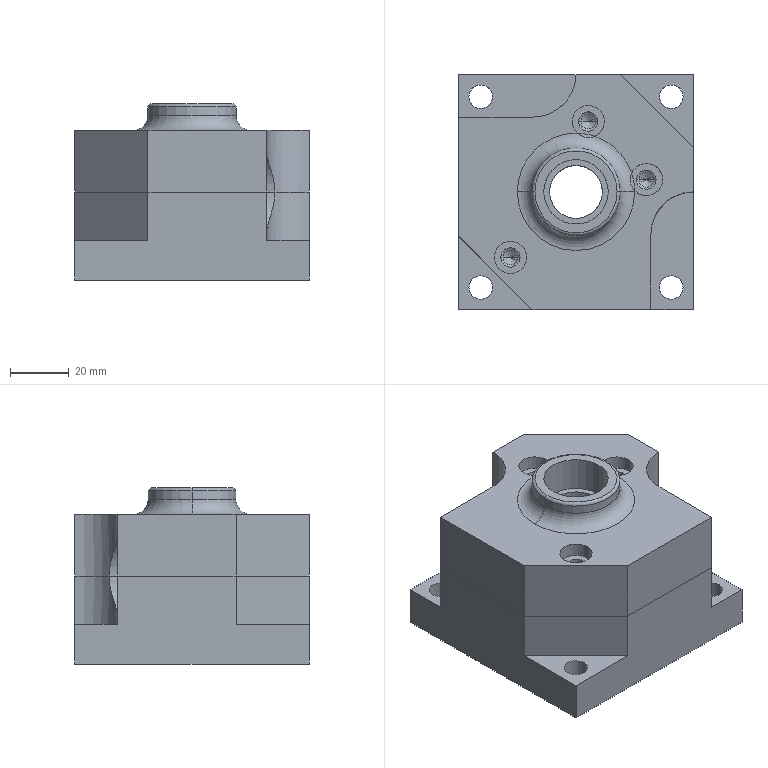Part | SolidWorks | features BaseBody 4 | 4 solids | 154 faces | box 80 x 80 x 60 mm | volume 202801 mm3 | cylinder 76 | plane 58 | cone 12 | torus 8 | commonest cylinder face diameters 28 x12 4 x8 8 x8 5 x6 6.6 x6 11 x6